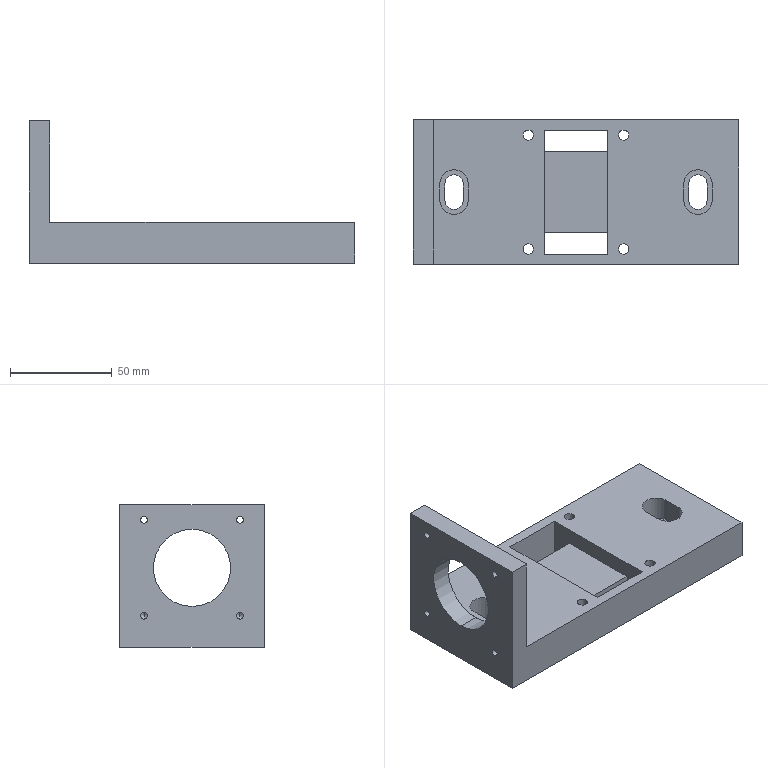Part | 1 solid | 55 faces | box 160 x 71 x 70 mm | volume 217862 mm3 | cylinder 26 | plane 25 | cone 4 | commonest cylinder face diameters 3.3 x8 5 x8 9 x4 14 x4 38 x2